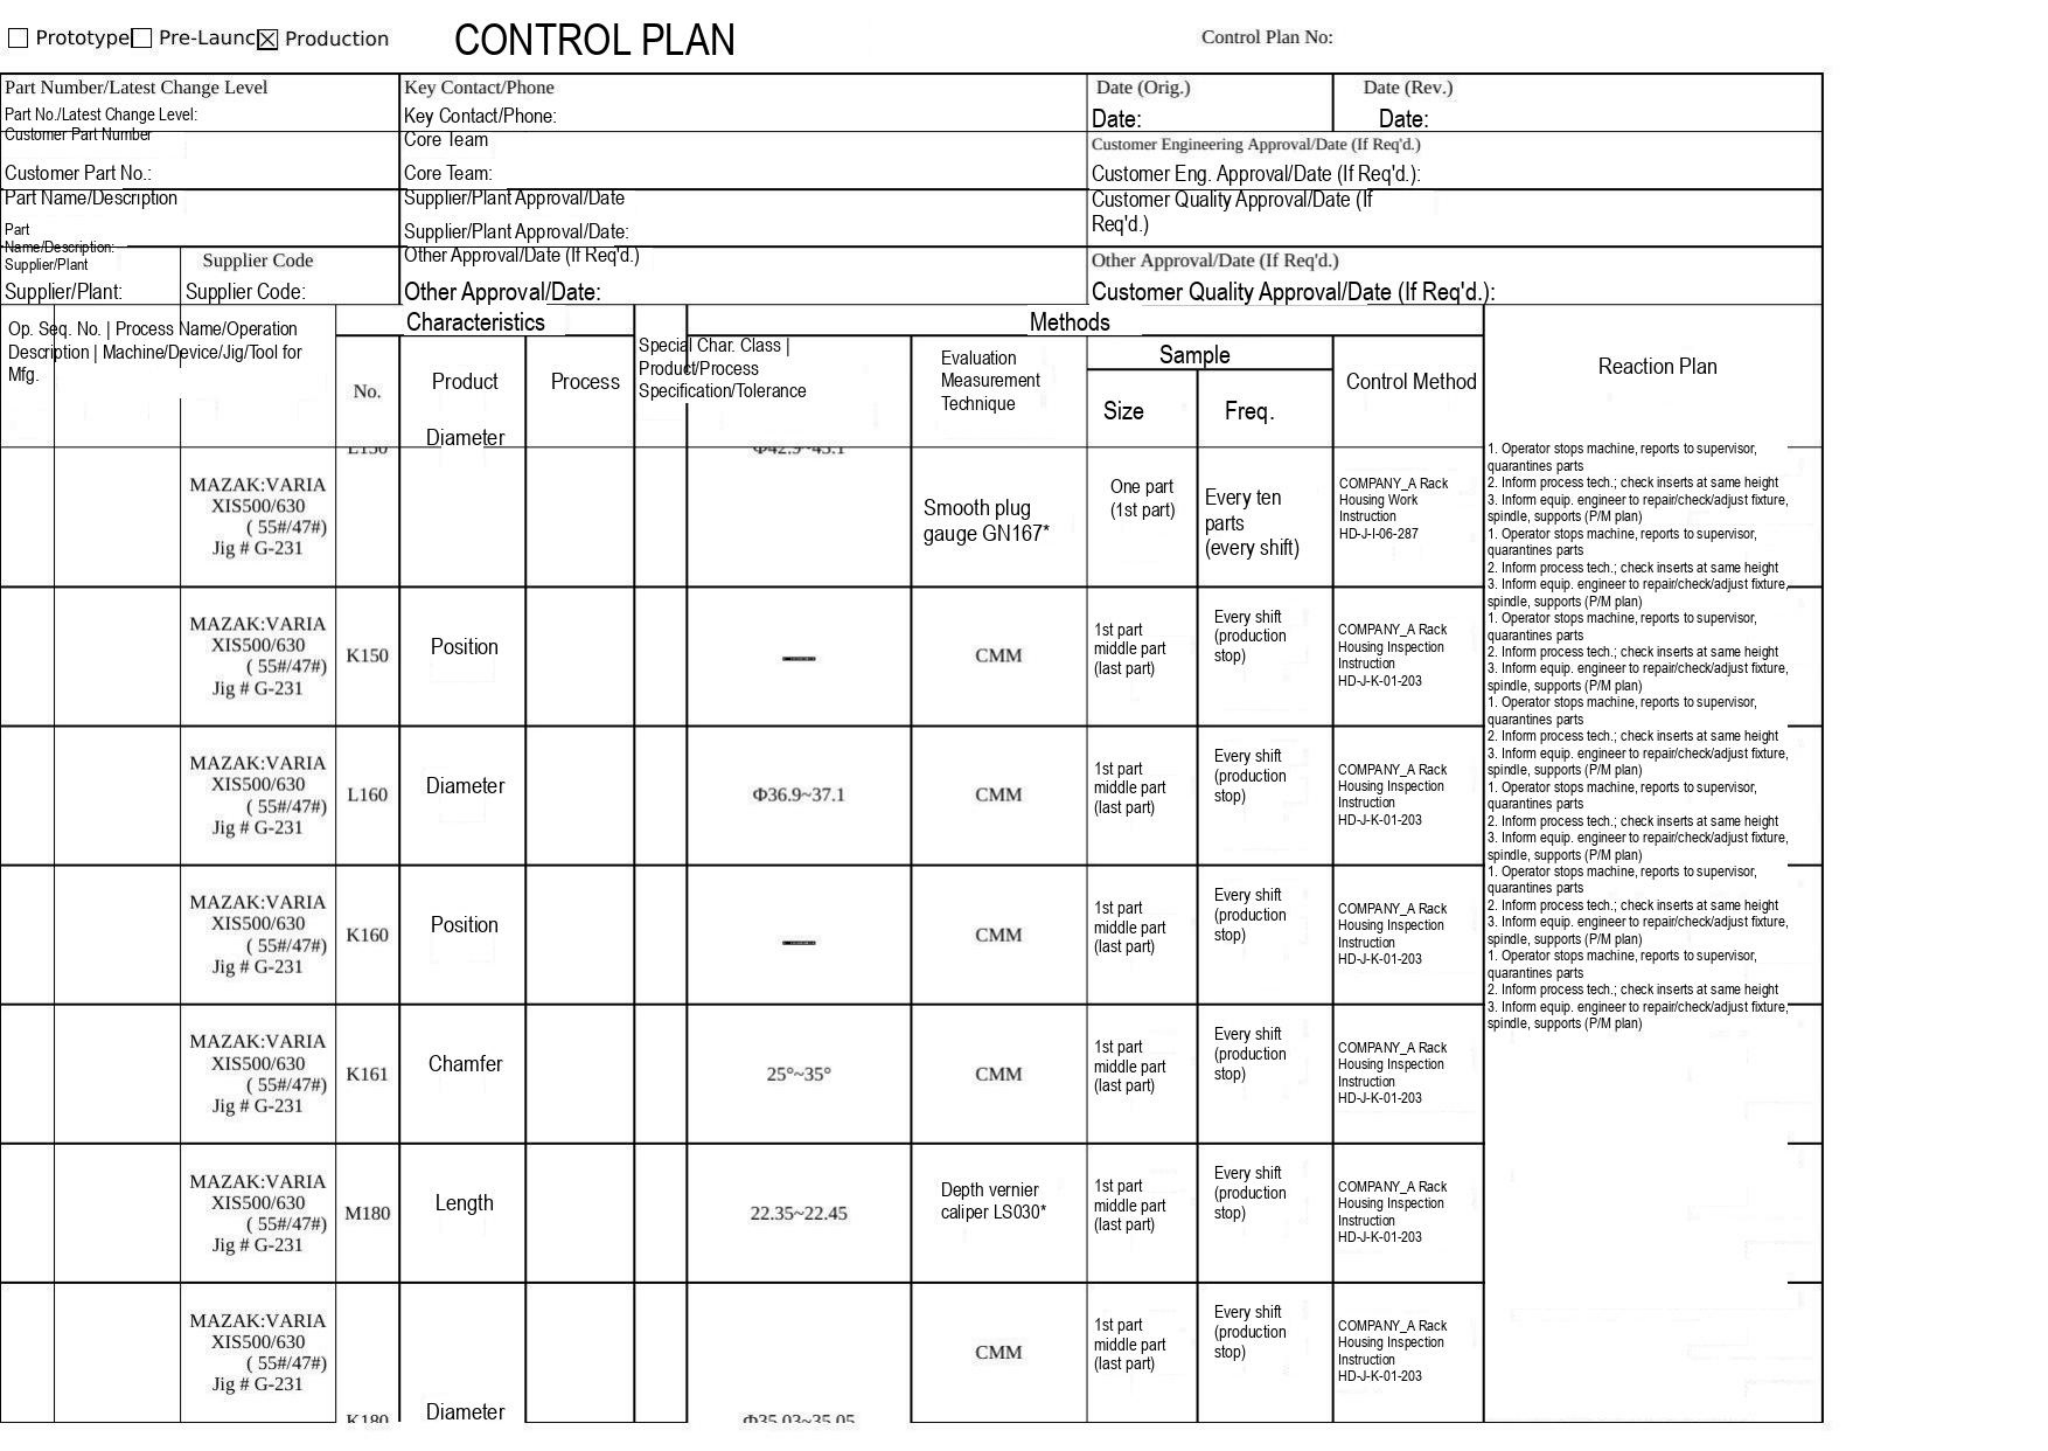☐ Prototype☐ Pre-Launc☒ Production

# CONTROL PLAN

Control Plan No:

| Part Number/Latest Change Level | | Key Contact/Phone | Date (Orig.) | Date (Rev.) |
|---|---|---|---|---|
| Part No./Latest Change Level: | | Key Contact/Phone: | Date: | Date: |
| Customer Part Number | | Core Team | Customer Engineering Approval/Date (If Req'd.) | |
| Customer Part No.: | | Core Team: | Customer Eng. Approval/Date (If Req'd.): | |
| Part Name/Description | | Supplier/Plant Approval/Date | Customer Quality Approval/Date (If Req'd.) | |
| Part Name/Description: | | Supplier/Plant Approval/Date: | | |
| Supplier/Plant | Supplier Code | Other Approval/Date (If Req'd.) | Other Approval/Date (If Req'd.) | |
| Supplier/Plant: | Supplier Code: | Other Approval/Date: | Customer Quality Approval/Date (If Req'd.): | |

| Op. Seq. No. | Process Name/Operation Description | Machine/Device/Jig/Tool for Mfg. | Characteristics No. | Characteristics Product | Characteristics Process | Special Char. Class | Product/Process Specification/Tolerance | Methods Evaluation Measurement Technique | Methods Sample Size | Methods Sample Freq. | Methods Control Method | Reaction Plan |
|---|---|---|---|---|---|---|---|---|---|---|---|---|
| | | MAZAK:VARIA XIS500/630 ( 55#/47#) Jig # G-231 | | Diameter | | | | Smooth plug gauge GN167* | One part (1st part) | Every ten parts (every shift) | COMPANY_A Rack Housing Work Instruction HD-J-I-06-287 | 1. Operator stops machine, reports to supervisor, quarantines parts 2. Inform process tech.; check inserts at same height 3. Inform equip. engineer to repair/check/adjust fixture, spindle, supports (P/M plan) |
| | | MAZAK:VARIA XIS500/630 ( 55#/47#) Jig # G-231 | K150 | Position | | | — | CMM | 1st part middle part (last part) | Every shift (production stop) | COMPANY_A Rack Housing Inspection Instruction HD-J-K-01-203 | 1. Operator stops machine, reports to supervisor, quarantines parts 2. Inform process tech.; check inserts at same height 3. Inform equip. engineer to repair/check/adjust fixture, spindle, supports (P/M plan) |
| | | MAZAK:VARIA XIS500/630 ( 55#/47#) Jig # G-231 | L160 | Diameter | | | Φ36.9~37.1 | CMM | 1st part middle part (last part) | Every shift (production stop) | COMPANY_A Rack Housing Inspection Instruction HD-J-K-01-203 | 1. Operator stops machine, reports to supervisor, quarantines parts 2. Inform process tech.; check inserts at same height 3. Inform equip. engineer to repair/check/adjust fixture, spindle, supports (P/M plan) |
| | | MAZAK:VARIA XIS500/630 ( 55#/47#) Jig # G-231 | K160 | Position | | | — | CMM | 1st part middle part (last part) | Every shift (production stop) | COMPANY_A Rack Housing Inspection Instruction HD-J-K-01-203 | 1. Operator stops machine, reports to supervisor, quarantines parts 2. Inform process tech.; check inserts at same height 3. Inform equip. engineer to repair/check/adjust fixture, spindle, supports (P/M plan) |
| | | MAZAK:VARIA XIS500/630 ( 55#/47#) Jig # G-231 | K161 | Chamfer | | | 25°~35° | CMM | 1st part middle part (last part) | Every shift (production stop) | COMPANY_A Rack Housing Inspection Instruction HD-J-K-01-203 | 1. Operator stops machine, reports to supervisor, quarantines parts 2. Inform process tech.; check inserts at same height 3. Inform equip. engineer to repair/check/adjust fixture, spindle, supports (P/M plan) |
| | | MAZAK:VARIA XIS500/630 ( 55#/47#) Jig # G-231 | M180 | Length | | | 22.35~22.45 | Depth vernier caliper LS030* | 1st part middle part (last part) | Every shift (production stop) | COMPANY_A Rack Housing Inspection Instruction HD-J-K-01-203 | 1. Operator stops machine, reports to supervisor, quarantines parts 2. Inform process tech.; check inserts at same height 3. Inform equip. engineer to repair/check/adjust fixture, spindle, supports (P/M plan) |
| | | MAZAK:VARIA XIS500/630 ( 55#/47#) Jig # G-231 | K180 | Diameter | | | Φ35.03~35.05 | CMM | 1st part middle part (last part) | Every shift (production stop) | COMPANY_A Rack Housing Inspection Instruction HD-J-K-01-203 | 1. Operator stops machine, reports to supervisor, quarantines parts 2. Inform process tech.; check inserts at same height 3. Inform equip. engineer to repair/check/adjust fixture, spindle, supports (P/M plan) |
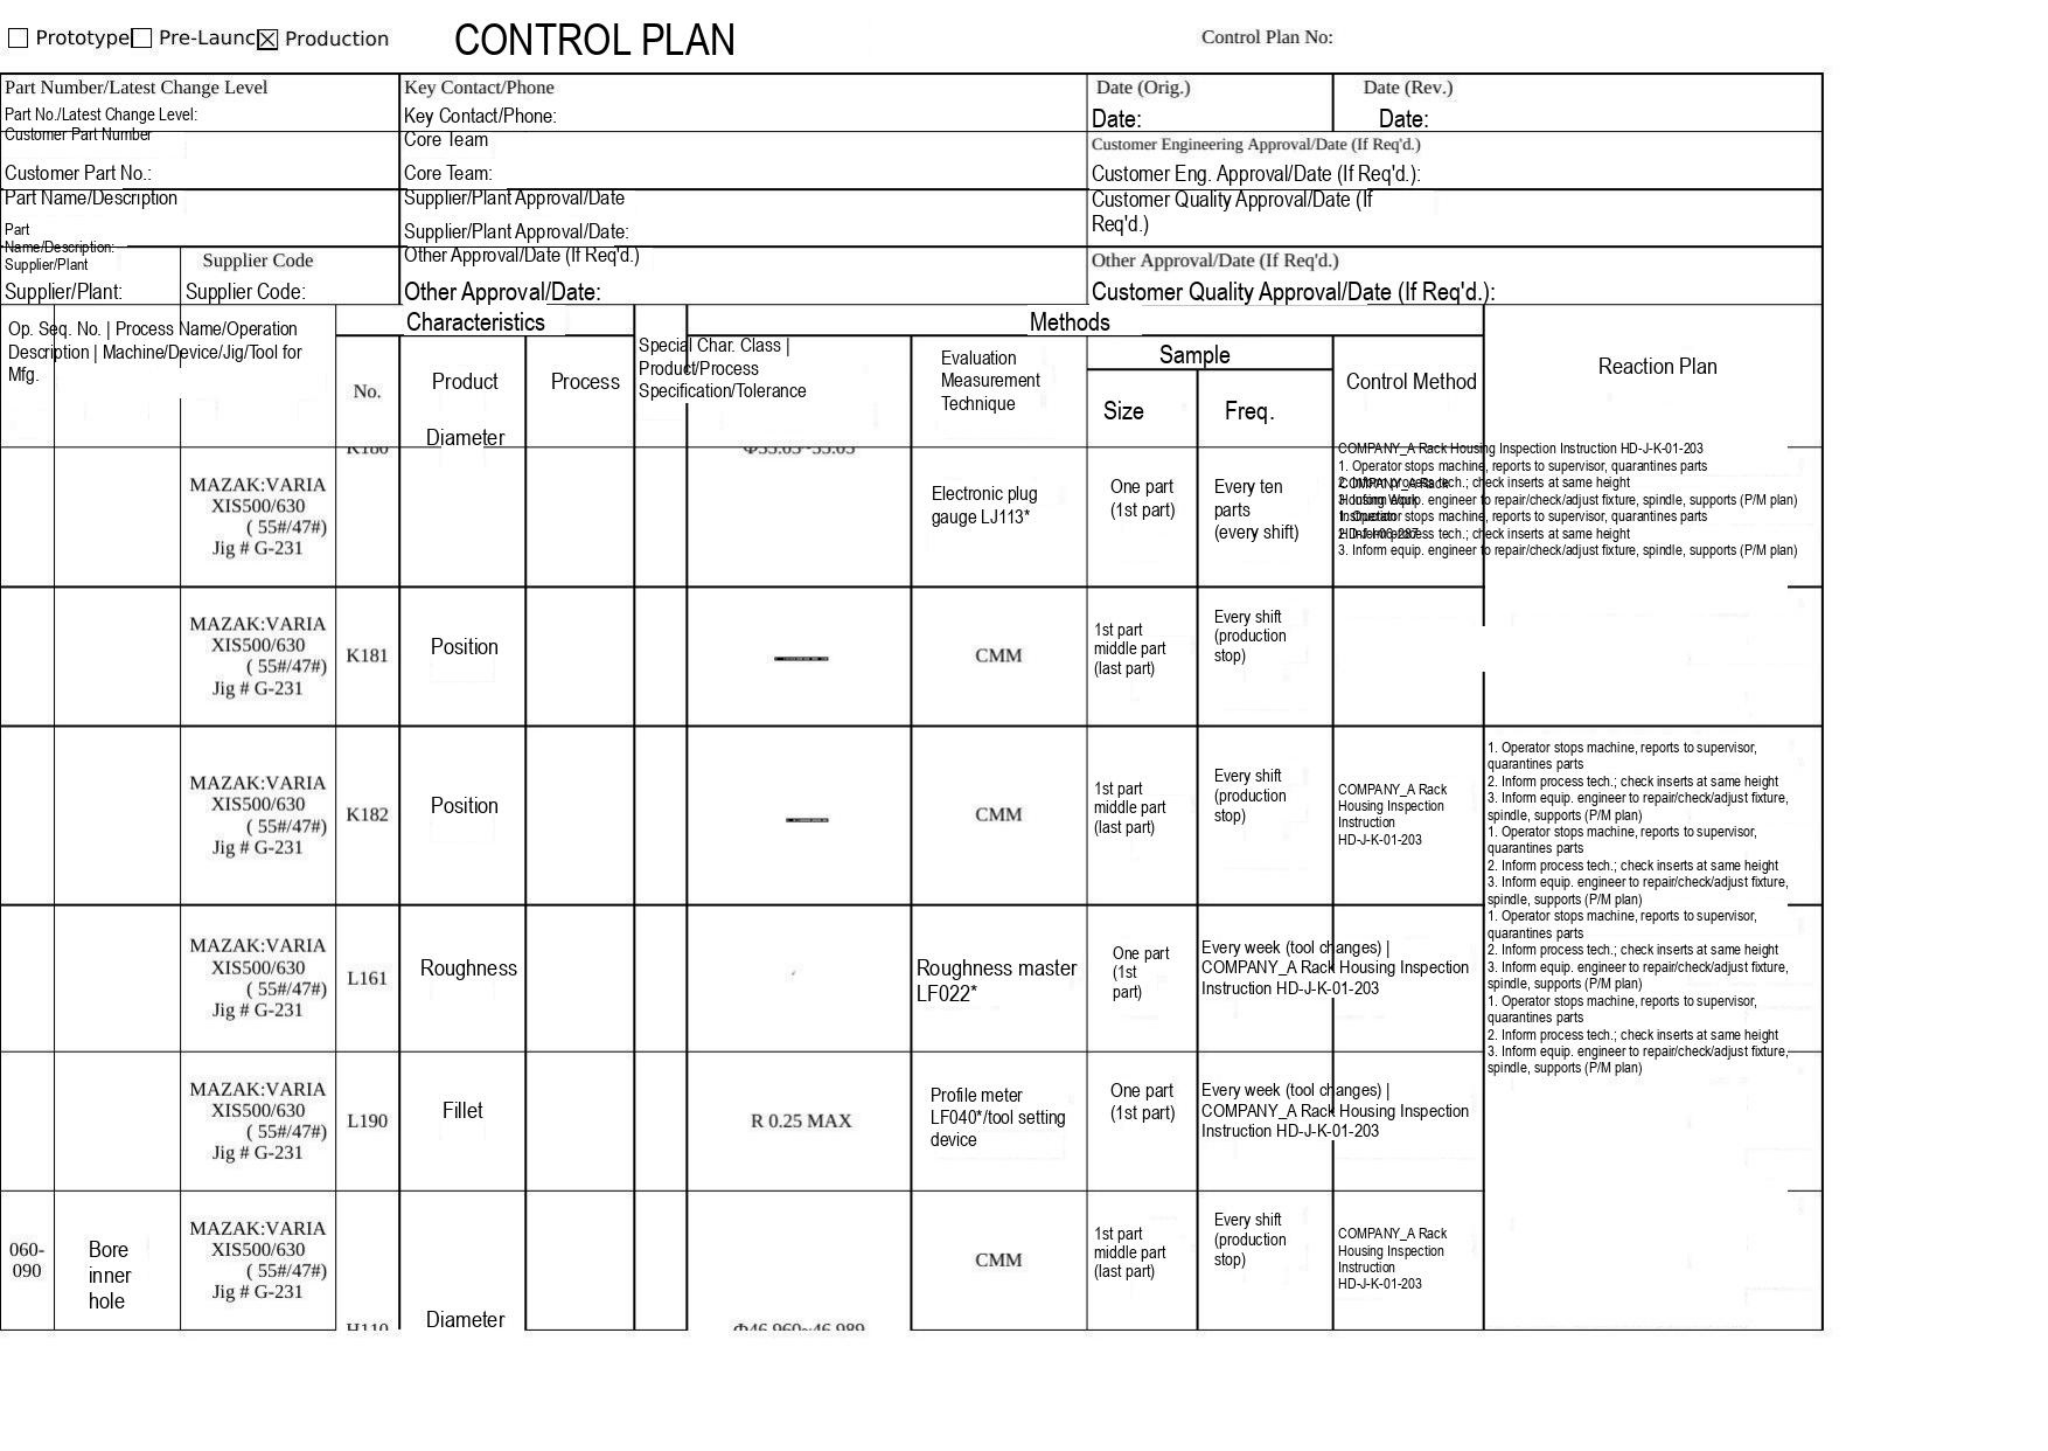☐ Prototype ☐ Pre-Launch ☒ Production

CONTROL PLAN

Control Plan No:

| Part Number/Latest Change Level<br>Part No./Latest Change Level: | Key Contact/Phone<br>Key Contact/Phone: | Date (Orig.)<br>Date: | Date (Rev.)<br>Date: |
|---|---|---|---|
| Customer Part Number<br>Customer Part No.: | Core Team<br>Core Team: | Customer Engineering Approval/Date (If Req'd.)<br>Customer Eng. Approval/Date (If Req'd.): | |
| Part Name/Description<br>Part Name/Description: | Supplier/Plant Approval/Date<br>Supplier/Plant Approval/Date: | Customer Quality Approval/Date (If Req'd.) | |
| Supplier/Plant<br>Supplier/Plant: Supplier Code<br>Supplier Code: | Other Approval/Date (If Req'd.)<br>Other Approval/Date: | Other Approval/Date (If Req'd.)<br>Customer Quality Approval/Date (If Req'd.): | |

| Op. Seq. No. \| Process Name/Operation Description \| Machine/Device/Jig/Tool for Mfg. | | | Characteristics No. | Characteristics Product | Characteristics Process | Special Char. Class \| Product/Process Specification/Tolerance | | Methods Evaluation Measurement Technique | Sample Size | Sample Freq. | Control Method | Reaction Plan |
|---|---|---|---|---|---|---|---|---|---|---|---|---|
| | | MAZAK:VARIA XIS500/630 ( 55#/47#) Jig # G-231 | K180 | Diameter | | | Φ55.65~55.65 | Electronic plug gauge LJ113* | One part (1st part) | Every ten parts (every shift) | COMPANY_A Rack Housing Inspection Instruction HD-J-K-01-203 | 1. Operator stops machine, reports to supervisor, quarantines parts<br>2. Inform process tech.; check inserts at same height<br>3. Inform equip. engineer to repair/check/adjust fixture, spindle, supports (P/M plan)<br>1. Operator stops machine, reports to supervisor, quarantines parts<br>2. Inform process tech.; check inserts at same height<br>3. Inform equip. engineer to repair/check/adjust fixture, spindle, supports (P/M plan) |
| | | MAZAK:VARIA XIS500/630 ( 55#/47#) Jig # G-231 | K181 | Position | | | | CMM | 1st part middle part (last part) | Every shift (production stop) | | |
| | | MAZAK:VARIA XIS500/630 ( 55#/47#) Jig # G-231 | K182 | Position | | | | CMM | 1st part middle part (last part) | Every shift (production stop) | COMPANY_A Rack Housing Inspection Instruction HD-J-K-01-203 | 1. Operator stops machine, reports to supervisor, quarantines parts<br>2. Inform process tech.; check inserts at same height<br>3. Inform equip. engineer to repair/check/adjust fixture, spindle, supports (P/M plan)<br>1. Operator stops machine, reports to supervisor, quarantines parts<br>2. Inform process tech.; check inserts at same height<br>3. Inform equip. engineer to repair/check/adjust fixture, spindle, supports (P/M plan)<br>1. Operator stops machine, reports to supervisor, quarantines parts<br>2. Inform process tech.; check inserts at same height<br>3. Inform equip. engineer to repair/check/adjust fixture, spindle, supports (P/M plan)<br>1. Operator stops machine, reports to supervisor, quarantines parts<br>2. Inform process tech.; check inserts at same height<br>3. Inform equip. engineer to repair/check/adjust fixture, spindle, supports (P/M plan) |
| | | MAZAK:VARIA XIS500/630 ( 55#/47#) Jig # G-231 | L161 | Roughness | | | | Roughness master LF022* | One part (1st part) | Every week (tool changes) \| COMPANY_A Rack Housing Inspection Instruction HD-J-K-01-203 | | |
| | | MAZAK:VARIA XIS500/630 ( 55#/47#) Jig # G-231 | L190 | Fillet | | | R 0.25 MAX | Profile meter LF040*/tool setting device | One part (1st part) | Every week (tool changes) \| COMPANY_A Rack Housing Inspection Instruction HD-J-K-01-203 | | |
| 060-090 | Bore inner hole | MAZAK:VARIA XIS500/630 ( 55#/47#) Jig # G-231 | H110 | Diameter | | | Φ46.960~46.989 | CMM | 1st part middle part (last part) | Every shift (production stop) | COMPANY_A Rack Housing Inspection Instruction HD-J-K-01-203 | |
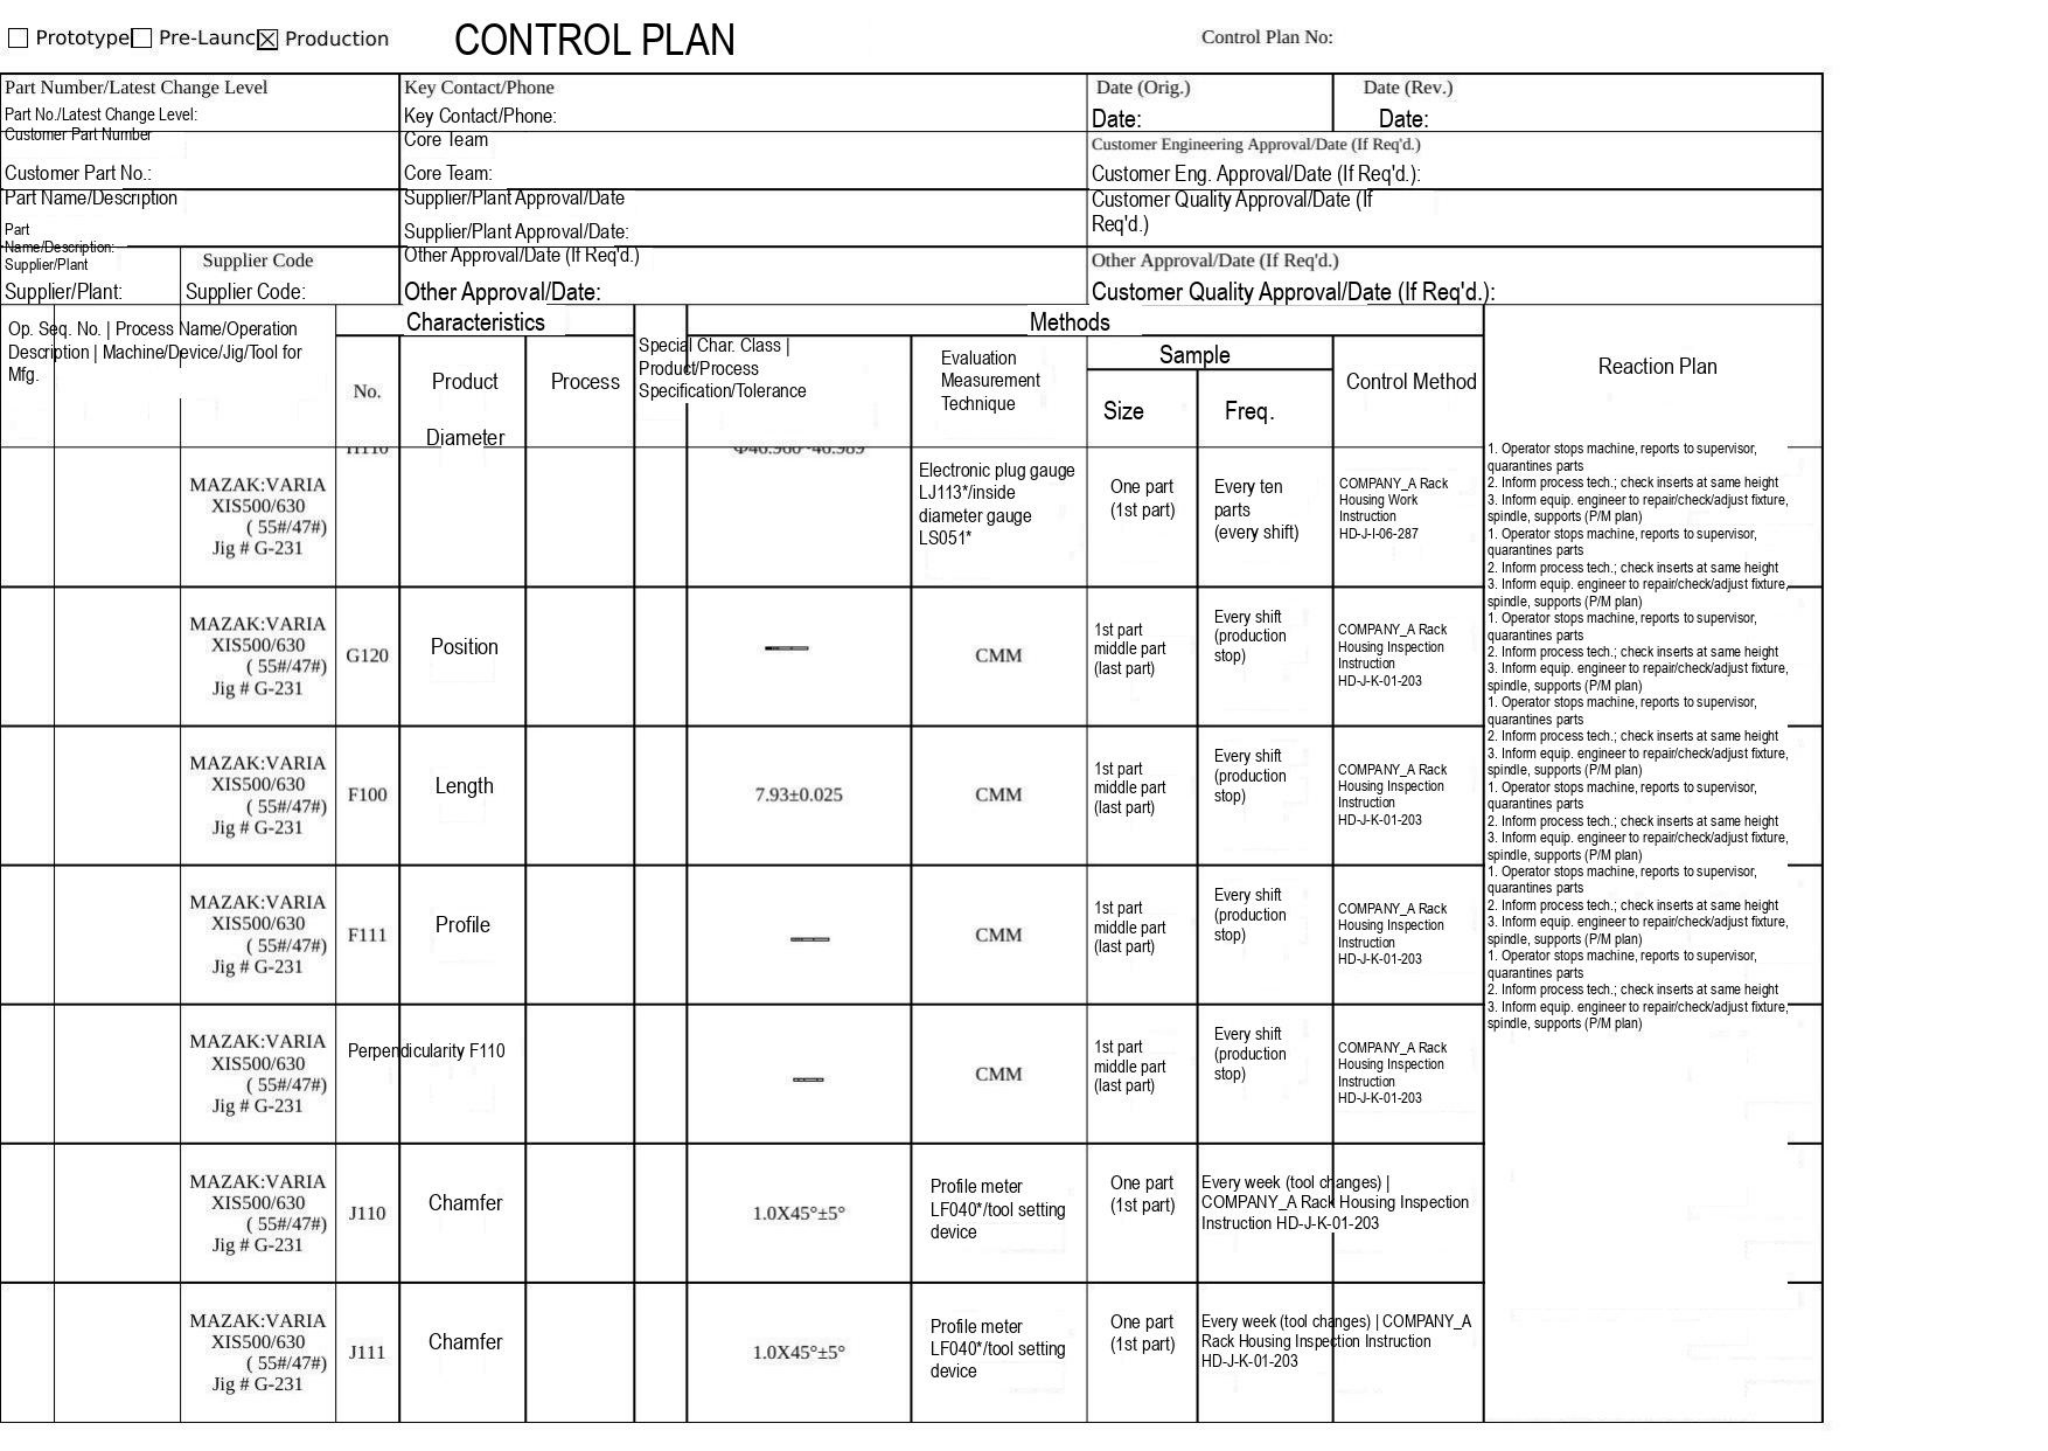☐ Prototype☐ Pre-Launc☒ Production

# CONTROL PLAN

Control Plan No:

| Part Number/Latest Change Level | Key Contact/Phone | Date (Orig.) | Date (Rev.) |
|---|---|---|---|
| Part No./Latest Change Level: | Key Contact/Phone: | Date: | Date: |
| Customer Part Number | Core Team | Customer Engineering Approval/Date (If Req'd.) | |
| Customer Part No.: | Core Team: | Customer Eng. Approval/Date (If Req'd.): | |
| Part Name/Description | Supplier/Plant Approval/Date | Customer Quality Approval/Date (If Req'd.) | |
| Part Name/Description: | Supplier/Plant Approval/Date: | | |

| Supplier/Plant | Supplier Code | Other Approval/Date (If Req'd.) | Other Approval/Date (If Req'd.) |
|---|---|---|---|
| Supplier/Plant: | Supplier Code: | Other Approval/Date: | Customer Quality Approval/Date (If Req'd.): |

| Op. Seq. No. | Process Name/Operation Description | Machine/Device/Jig/Tool for Mfg. | Characteristics | | | Methods | | | | | | Reaction Plan |
|---|---|---|---|---|---|---|---|---|---|---|---|---|
| | | | No. | Product | Process | Special Char. Class | Product/Process Specification/Tolerance | Evaluation Measurement Technique | Sample Size | Sample Freq. | Control Method | |
| | | MAZAK:VARIA XIS500/630 ( 55#/47#) Jig # G-231 | H110 | Diameter | | | Φ46.960-46.989 | Electronic plug gauge LJ113*/inside diameter gauge LS051* | One part (1st part) | Every ten parts (every shift) | COMPANY_A Rack Housing Work Instruction HD-J-I-06-287 | 1. Operator stops machine, reports to supervisor, quarantines parts 2. Inform process tech.; check inserts at same height 3. Inform equip. engineer to repair/check/adjust fixture, spindle, supports (P/M plan) |
| | | MAZAK:VARIA XIS500/630 ( 55#/47#) Jig # G-231 | G120 | Position | | | — | CMM | 1st part middle part (last part) | Every shift (production stop) | COMPANY_A Rack Housing Inspection Instruction HD-J-K-01-203 | 1. Operator stops machine, reports to supervisor, quarantines parts 2. Inform process tech.; check inserts at same height 3. Inform equip. engineer to repair/check/adjust fixture, spindle, supports (P/M plan) |
| | | MAZAK:VARIA XIS500/630 ( 55#/47#) Jig # G-231 | F100 | Length | | | 7.93±0.025 | CMM | 1st part middle part (last part) | Every shift (production stop) | COMPANY_A Rack Housing Inspection Instruction HD-J-K-01-203 | 1. Operator stops machine, reports to supervisor, quarantines parts 2. Inform process tech.; check inserts at same height 3. Inform equip. engineer to repair/check/adjust fixture, spindle, supports (P/M plan) |
| | | MAZAK:VARIA XIS500/630 ( 55#/47#) Jig # G-231 | F111 | Profile | | | — | CMM | 1st part middle part (last part) | Every shift (production stop) | COMPANY_A Rack Housing Inspection Instruction HD-J-K-01-203 | 1. Operator stops machine, reports to supervisor, quarantines parts 2. Inform process tech.; check inserts at same height 3. Inform equip. engineer to repair/check/adjust fixture, spindle, supports (P/M plan) |
| | | MAZAK:VARIA XIS500/630 ( 55#/47#) Jig # G-231 | Perpendicularity F110 | | | | — | CMM | 1st part middle part (last part) | Every shift (production stop) | COMPANY_A Rack Housing Inspection Instruction HD-J-K-01-203 | 1. Operator stops machine, reports to supervisor, quarantines parts 2. Inform process tech.; check inserts at same height 3. Inform equip. engineer to repair/check/adjust fixture, spindle, supports (P/M plan) |
| | | MAZAK:VARIA XIS500/630 ( 55#/47#) Jig # G-231 | J110 | Chamfer | | | 1.0X45°±5° | Profile meter LF040*/tool setting device | One part (1st part) | Every week (tool changes) \| COMPANY_A Rack Housing Inspection Instruction HD-J-K-01-203 | | 1. Operator stops machine, reports to supervisor, quarantines parts 2. Inform process tech.; check inserts at same height 3. Inform equip. engineer to repair/check/adjust fixture, spindle, supports (P/M plan) |
| | | MAZAK:VARIA XIS500/630 ( 55#/47#) Jig # G-231 | J111 | Chamfer | | | 1.0X45°±5° | Profile meter LF040*/tool setting device | One part (1st part) | Every week (tool changes) \| COMPANY_A Rack Housing Inspection Instruction HD-J-K-01-203 | | 1. Operator stops machine, reports to supervisor, quarantines parts 2. Inform process tech.; check inserts at same height 3. Inform equip. engineer to repair/check/adjust fixture, spindle, supports (P/M plan) |
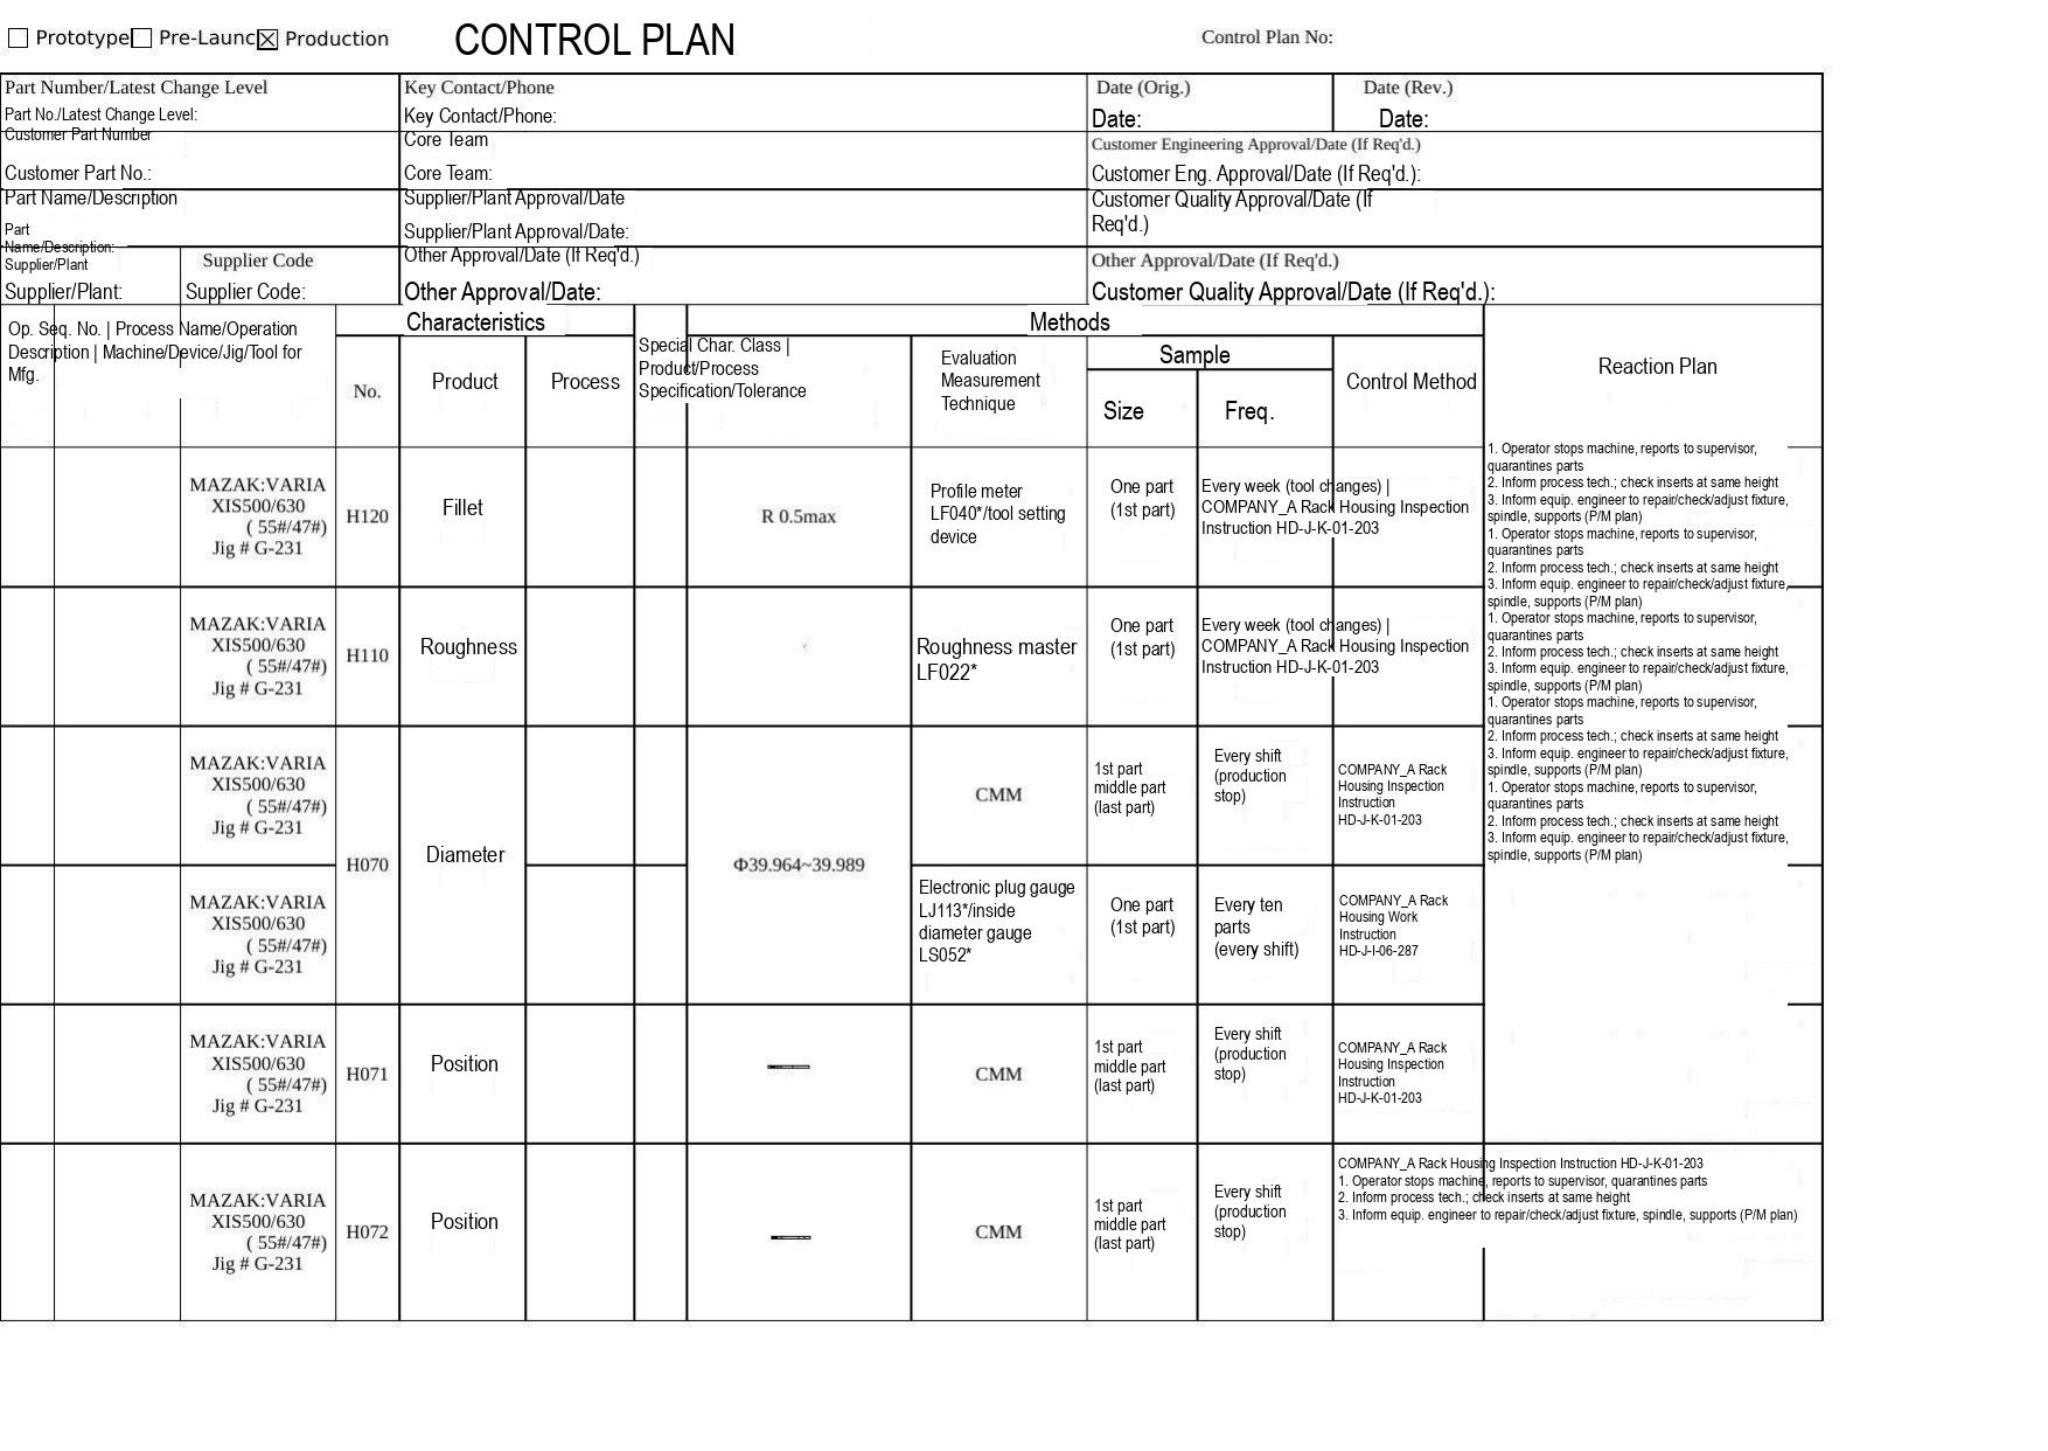☐ Prototype ☐ Pre-Launc ☒ Production

# CONTROL PLAN

Control Plan No:

| Part Number/Latest Change Level<br>Part No./Latest Change Level: | Key Contact/Phone<br>Key Contact/Phone: | Date (Orig.)<br>Date: | Date (Rev.)<br>Date: |
|---|---|---|---|
| Customer Part Number<br>Customer Part No.: | Core Team<br>Core Team: | Customer Engineering Approval/Date (If Req'd.)<br>Customer Eng. Approval/Date (If Req'd.): | |
| Part Name/Description<br>Part Name/Description: | Supplier/Plant Approval/Date<br>Supplier/Plant Approval/Date: | Customer Quality Approval/Date (If Req'd.) | |
| Supplier/Plant<br>Supplier/Plant: Supplier Code<br>Supplier Code: | Other Approval/Date (If Req'd.)<br>Other Approval/Date: | Other Approval/Date (If Req'd.)<br>Customer Quality Approval/Date (If Req'd.): | |

| Op. Seq. No. | Process Name/Operation Description | Machine/Device/Jig/Tool for Mfg. | Characteristics No. | Characteristics Product | Characteristics Process | Special Char. Class | Product/Process Specification/Tolerance | Methods Evaluation Measurement Technique | Sample Size | Sample Freq. | Control Method | Reaction Plan |
|---|---|---|---|---|---|---|---|---|---|---|---|---|
| | | MAZAK:VARIA XIS500/630 ( 55#/47#) Jig # G-231 | H120 | Fillet | | | R 0.5max | Profile meter LF040*/tool setting device | One part (1st part) | Every week (tool changes) | | COMPANY_A Rack Housing Inspection Instruction HD-J-K-01-203 | 1. Operator stops machine, reports to supervisor, quarantines parts<br>2. Inform process tech.; check inserts at same height<br>3. Inform equip. engineer to repair/check/adjust fixture, spindle, supports (P/M plan)<br>1. Operator stops machine, reports to supervisor, quarantines parts<br>2. Inform process tech.; check inserts at same height<br>3. Inform equip. engineer to repair/check/adjust fixture, spindle, supports (P/M plan) |
| | | MAZAK:VARIA XIS500/630 ( 55#/47#) Jig # G-231 | H110 | Roughness | | | | Roughness master LF022* | One part (1st part) | Every week (tool changes) | | COMPANY_A Rack Housing Inspection Instruction HD-J-K-01-203 | 1. Operator stops machine, reports to supervisor, quarantines parts<br>2. Inform process tech.; check inserts at same height<br>3. Inform equip. engineer to repair/check/adjust fixture, spindle, supports (P/M plan)<br>1. Operator stops machine, reports to supervisor, quarantines parts<br>2. Inform process tech.; check inserts at same height<br>3. Inform equip. engineer to repair/check/adjust fixture, spindle, supports (P/M plan) |
| | | MAZAK:VARIA XIS500/630 ( 55#/47#) Jig # G-231 | H070 | Diameter | | | Φ39.964~39.989 | CMM | 1st part middle part (last part) | Every shift (production stop) | COMPANY_A Rack Housing Inspection Instruction HD-J-K-01-203 | 1. Operator stops machine, reports to supervisor, quarantines parts<br>2. Inform process tech.; check inserts at same height<br>3. Inform equip. engineer to repair/check/adjust fixture, spindle, supports (P/M plan) |
| | | MAZAK:VARIA XIS500/630 ( 55#/47#) Jig # G-231 | H070 | Diameter | | | Φ39.964~39.989 | Electronic plug gauge LJ113*/inside diameter gauge LS052* | One part (1st part) | Every ten parts (every shift) | COMPANY_A Rack Housing Work Instruction HD-J-I-06-287 | |
| | | MAZAK:VARIA XIS500/630 ( 55#/47#) Jig # G-231 | H071 | Position | | | | CMM | 1st part middle part (last part) | Every shift (production stop) | COMPANY_A Rack Housing Inspection Instruction HD-J-K-01-203 | |
| | | MAZAK:VARIA XIS500/630 ( 55#/47#) Jig # G-231 | H072 | Position | | | | CMM | 1st part middle part (last part) | Every shift (production stop) | COMPANY_A Rack Housing Inspection Instruction HD-J-K-01-203 | 1. Operator stops machine, reports to supervisor, quarantines parts<br>2. Inform process tech.; check inserts at same height<br>3. Inform equip. engineer to repair/check/adjust fixture, spindle, supports (P/M plan) |
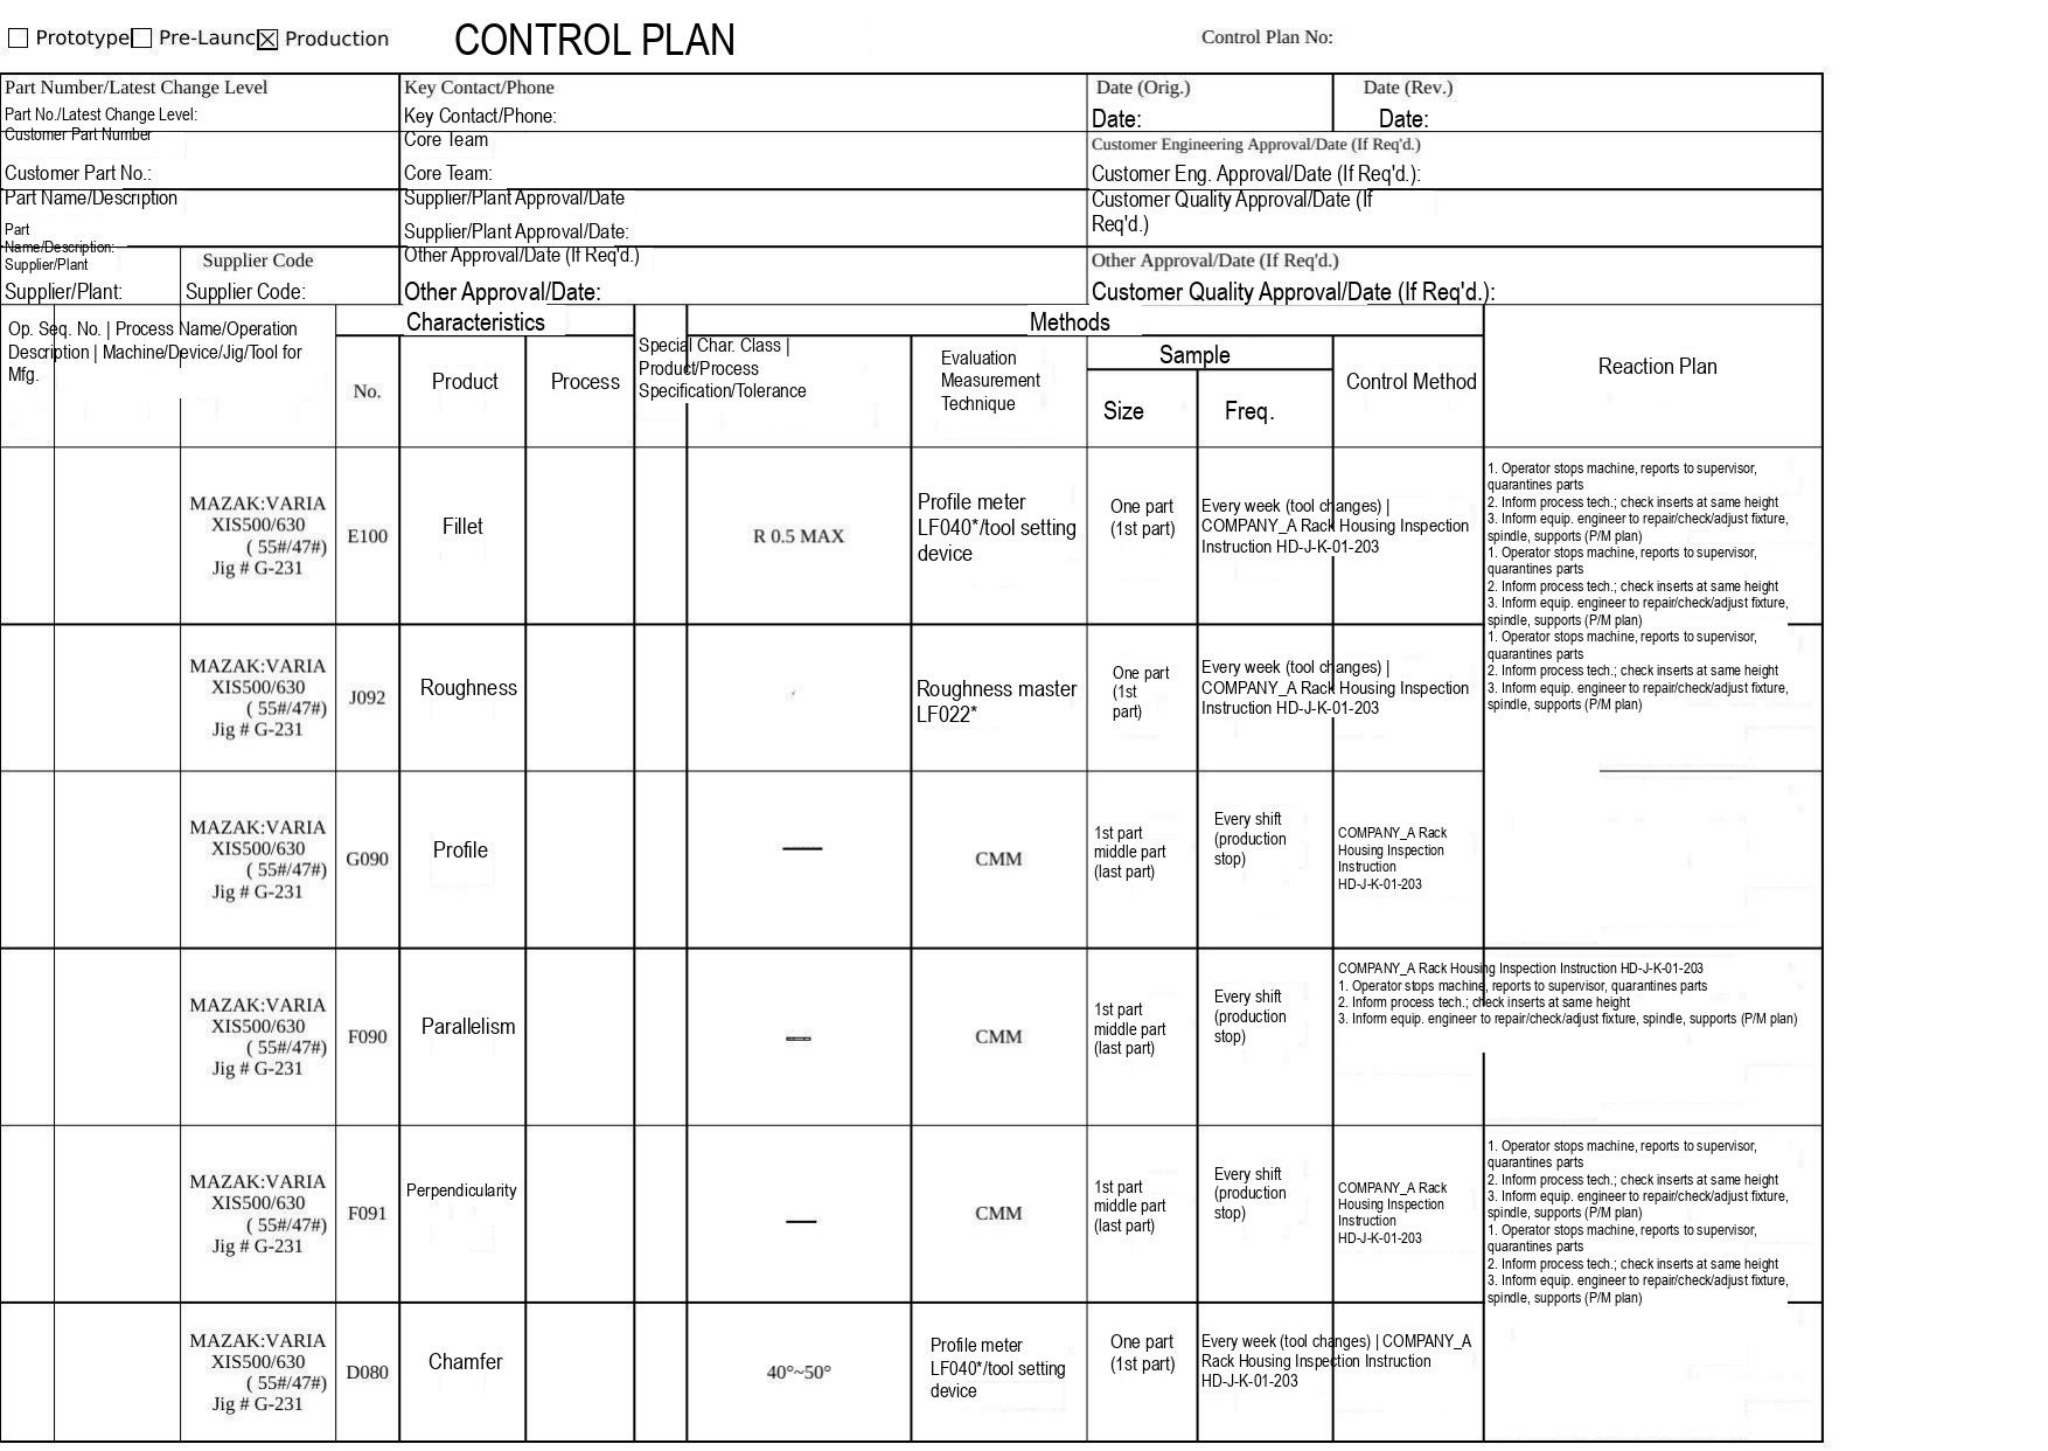☐ Prototype☐ Pre-Launc☒ Production

CONTROL PLAN

Control Plan No:

| Part Number/Latest Change Level<br>Part No./Latest Change Level: | | Key Contact/Phone<br>Key Contact/Phone: | Date (Orig.)<br>Date: | Date (Rev.)<br>Date: |
|---|---|---|---|---|
| Customer Part Number<br>Customer Part No.: | | Core Team<br>Core Team: | Customer Engineering Approval/Date (If Req'd.)<br>Customer Eng. Approval/Date (If Req'd.): | |
| Part Name/Description<br>Part Name/Description: | | Supplier/Plant Approval/Date<br>Supplier/Plant Approval/Date: | Customer Quality Approval/Date (If Req'd.) | |
| Supplier/Plant<br>Supplier/Plant: | Supplier Code<br>Supplier Code: | Other Approval/Date (If Req'd.)<br>Other Approval/Date: | Other Approval/Date (If Req'd.)<br>Customer Quality Approval/Date (If Req'd.): | |

| Op. Seq. No. \| Process Name/Operation Description \| Machine/Device/Jig/Tool for Mfg. | | | Characteristics No. | Characteristics Product | Characteristics Process | Special Char. Class \| Product/Process Specification/Tolerance | | Methods Evaluation Measurement Technique | Methods Sample Size | Methods Sample Freq. | Methods Control Method | Reaction Plan |
|---|---|---|---|---|---|---|---|---|---|---|---|---|
| | | MAZAK:VARIA XIS500/630 ( 55#/47#) Jig # G-231 | E100 | Fillet | | | R 0.5 MAX | Profile meter LF040*/tool setting device | One part (1st part) | Every week (tool changes) \| COMPANY_A Rack Housing Inspection Instruction HD-J-K-01-203 | | 1. Operator stops machine, reports to supervisor, quarantines parts<br>2. Inform process tech.; check inserts at same height<br>3. Inform equip. engineer to repair/check/adjust fixture, spindle, supports (P/M plan)<br>1. Operator stops machine, reports to supervisor, quarantines parts<br>2. Inform process tech.; check inserts at same height<br>3. Inform equip. engineer to repair/check/adjust fixture, spindle, supports (P/M plan) |
| | | MAZAK:VARIA XIS500/630 ( 55#/47#) Jig # G-231 | J092 | Roughness | | | | Roughness master LF022* | One part (1st part) | Every week (tool changes) \| COMPANY_A Rack Housing Inspection Instruction HD-J-K-01-203 | | 1. Operator stops machine, reports to supervisor, quarantines parts<br>2. Inform process tech.; check inserts at same height<br>3. Inform equip. engineer to repair/check/adjust fixture, spindle, supports (P/M plan) |
| | | MAZAK:VARIA XIS500/630 ( 55#/47#) Jig # G-231 | G090 | Profile | | | — | CMM | 1st part middle part (last part) | Every shift (production stop) | COMPANY_A Rack Housing Inspection Instruction HD-J-K-01-203 | |
| | | MAZAK:VARIA XIS500/630 ( 55#/47#) Jig # G-231 | F090 | Parallelism | | | — | CMM | 1st part middle part (last part) | Every shift (production stop) | COMPANY_A Rack Housing Inspection Instruction HD-J-K-01-203<br>1. Operator stops machine, reports to supervisor, quarantines parts<br>2. Inform process tech.; check inserts at same height<br>3. Inform equip. engineer to repair/check/adjust fixture, spindle, supports (P/M plan) | |
| | | MAZAK:VARIA XIS500/630 ( 55#/47#) Jig # G-231 | F091 | Perpendicularity | | | — | CMM | 1st part middle part (last part) | Every shift (production stop) | COMPANY_A Rack Housing Inspection Instruction HD-J-K-01-203 | 1. Operator stops machine, reports to supervisor, quarantines parts<br>2. Inform process tech.; check inserts at same height<br>3. Inform equip. engineer to repair/check/adjust fixture, spindle, supports (P/M plan)<br>1. Operator stops machine, reports to supervisor, quarantines parts<br>2. Inform process tech.; check inserts at same height<br>3. Inform equip. engineer to repair/check/adjust fixture, spindle, supports (P/M plan) |
| | | MAZAK:VARIA XIS500/630 ( 55#/47#) Jig # G-231 | D080 | Chamfer | | | 40°~50° | Profile meter LF040*/tool setting device | One part (1st part) | Every week (tool changes) \| COMPANY_A Rack Housing Inspection Instruction HD-J-K-01-203 | | |